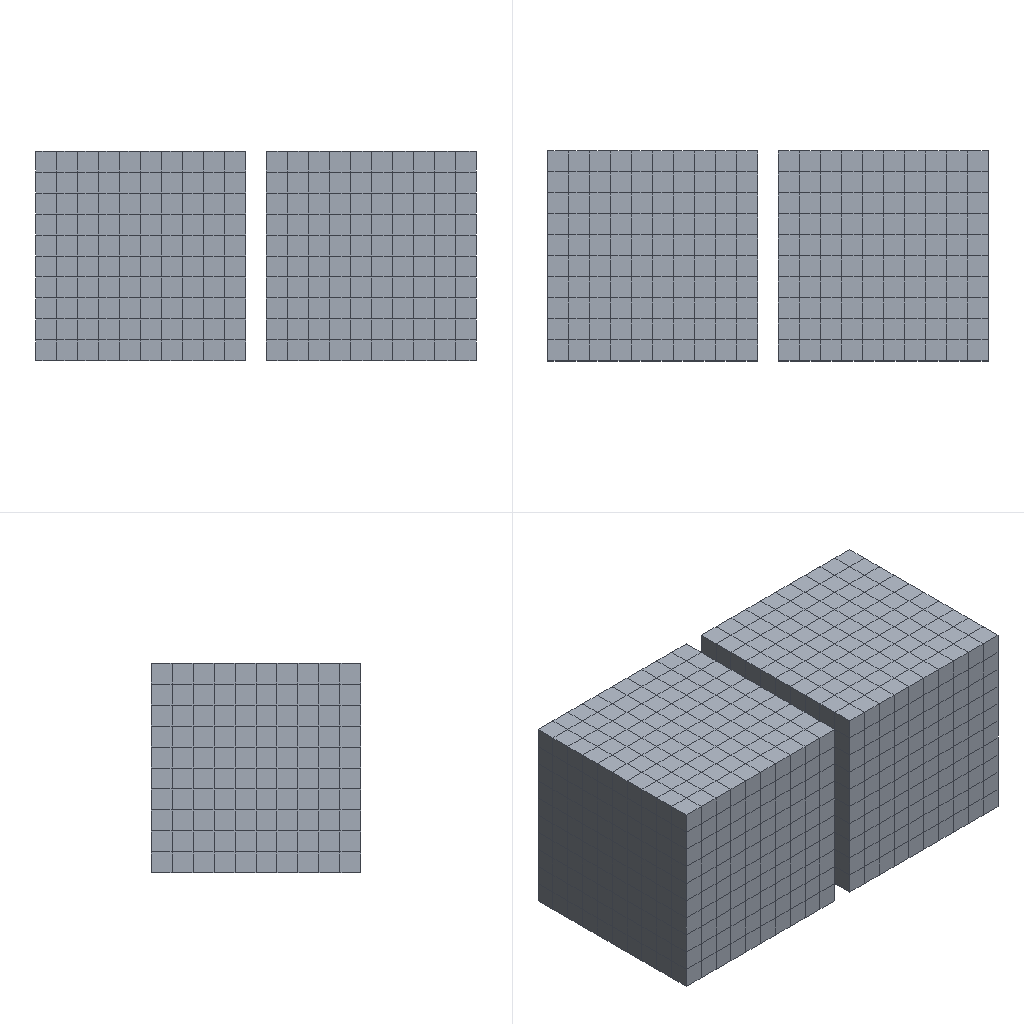Simulation study | abaqus
Set-up summary:
category,name,step,type,value,unit,region
solver,abaqus,,Abaqus/CAE 2024
units,SI m-kg-s (Pa),,inferred,E=3.45e+10 density=2550
analysis,Step-1,,frequency (modal),n_modes=10
mesh,nodes,,,2662
mesh,elements,,,2004
element_type,C3D8R,,,2000
element_type,CONN3D2,,,4
material,MATERIAL-1,,E,3.45e+10
material,MATERIAL-1,,nu,0.2
material,MATERIAL-1,,density,2550
material,MATERIAL-1,,behaviors,damping
material,MATERIAL-2,,E,3e+10
material,MATERIAL-2,,nu,0.3
material,MATERIAL-2,,density,2500
section,MATERIAL-2,,solid section,,,_PICKEDSET2
bc,Disp-BC-1,initial,encastre,[dofs=ENCASTRE],,_PICKEDSET37
constraint,connector section,,,1
Abaqus input file, long lists of numbers shortened:
*Heading
** Job name: deck Model name: 222
** Generated by: Abaqus/CAE 2024
*Preprint, echo=NO, model=NO, history=NO, contact=NO
**
** PARTS
**
*Part, name=PART-3
*Node
      1,          -5.,           0.,           5.
      2,          -5.,          0.5,           5.
** (1329 more lines like these left out)
*Element, type=C3D8R
   1,  122,  123,  134,  133,    1,    2,   13,   12
   2,  123,  124,  135,  134,    2,    3,   14,   13
** (998 more lines like these left out)
*Nset, nset=_PICKEDSET2, internal, generate
    1,  1331,     1
*Elset, elset=_PICKEDSET2, internal, generate
    1,  1000,     1
** Section: Section-1-_PICKEDSET2
*Solid Section, elset=_PICKEDSET2, material=MATERIAL-2
,
*End Part
**
**
** ASSEMBLY
**
*Assembly, name=Assembly
**
*Instance, name=PART-3-1, part=PART-3
*End Instance
**
*Instance, name=PART-3-2, part=PART-3
         5.5,           0.,           0.
*End Instance
**
*Element, type=CONN3D2
1, PART-3-1.122, PART-3-2.11
2, PART-3-1.133, PART-3-2.121
** (2 more lines like these left out)
*Connector Section, elset=_PickedSet21, behavior=ConnProp-1_CONNSECT-1
Cartesian, Cardan
"Datum csys-1",
*Nset, nset=SET-9, instance=PART-3-1
 1211, 1221, 1321, 1331
*Nset, nset=SET-9, instance=PART-3-2
   1,  11, 111, 121
*Nset, nset=WIRE-1-SET-3, instance=PART-3-1
 1211, 1221, 1321, 1331
*Nset, nset=WIRE-1-SET-3, instance=PART-3-2
   1,  11, 111, 121
*Nset, nset=_PICKEDSET32, internal, instance=PART-3-2, generate
 1211,  1331,     1
*Elset, elset=_PICKEDSET32, internal, instance=PART-3-2, generate
  901,  1000,     1
*Nset, nset=_PICKEDSET37, internal, instance=PART-3-2, generate
 1211,  1331,     1
*Elset, elset=_PICKEDSET37, internal, instance=PART-3-2, generate
  901,  1000,     1
*Elset, elset=_PickedSet21, internal, generate
 1,  4,  1
*Elset, elset=__PICKEDSURF33_S2, internal, instance=PART-3-1, generate
   1,  100,    1
*Surface, type=ELEMENT, name=_PICKEDSURF33, internal
__PICKEDSURF33_S2, S2
*Orientation, name="Datum csys-1"
          1.,           0.,           0.,           0.,           1.,           0.
1, 0.
*End Assembly
*Connector Behavior, name=ConnProp-1_CONNSECT-1
*Connector Elasticity, component=1
 5e+06,
*Connector Elasticity, component=2
 9e+09,
*Connector Elasticity, component=3
 6.9e+06,
**
** MATERIALS
**
*Material, name=MATERIAL-1
*Damping, alpha=0.516, beta=0.00077
*Density
2550.,
*Elastic
 3.45e+10, 0.2
*Material, name=MATERIAL-2
*Density
2500.,
*Elastic
 3e+10, 0.3
**
** BOUNDARY CONDITIONS
**
** Name: Disp-BC-1 Type: Symmetry/Antisymmetry/Encastre
*Boundary
_PICKEDSET37, ENCASTRE
** ----------------------------------------------------------------
**
** STEP: Step-1
**
*Step, name=Step-1, nlgeom=NO, perturbation
*Frequency, eigensolver=Lanczos, sim, acoustic coupling=on, normalization=mass
10, , , , ,
**
** OUTPUT REQUESTS
**
*Restart, write, frequency=0
**
** FIELD OUTPUT: F-Output-1
**
*Output, field
*Node Output
U,
*End Step
Results summary:
result,odb.job_status,,,JOB_STATUS_COMPLETED_SUCCESSFULLY,"consistent, unstated (Abaqus has no unit system)"
result,steps[0].procedure,Step-1,,*FREQUENCY,"consistent, unstated (Abaqus has no unit system)"
result,steps[0].time_period,Step-1,,0,"consistent, unstated (Abaqus has no unit system)"
result,steps[0].n_frames,Step-1,,11,"consistent, unstated (Abaqus has no unit system)"
result,steps[0].last_frame.id,Step-1,,1,"consistent, unstated (Abaqus has no unit system)"
result,steps[0].last_frame.value,Step-1,,10,"consistent, unstated (Abaqus has no unit system)"
result,steps[0].last_frame.description,Step-1,,Mode        10: Value =  6.75694E+05 Freq =   130.83     (cycles/time),"consistent, unstated (Abaqus has no unit system)"
result,steps[0].max_U_magnitude,Step-1,,0.003567,"consistent, unstated (Abaqus has no unit system)"
result,steps[0].eigenfrequencies_hz[1],Step-1,,0,"consistent, unstated (Abaqus has no unit system)"
result,steps[0].eigenfrequencies_hz[2],Step-1,,0,"consistent, unstated (Abaqus has no unit system)"
result,steps[0].eigenfrequencies_hz[3],Step-1,,0,"consistent, unstated (Abaqus has no unit system)"
result,steps[0].eigenfrequencies_hz[4],Step-1,,1.253,"consistent, unstated (Abaqus has no unit system)"
result,steps[0].eigenfrequencies_hz[5],Step-1,,1.522,"consistent, unstated (Abaqus has no unit system)"
result,steps[0].eigenfrequencies_hz[6],Step-1,,1.522,"consistent, unstated (Abaqus has no unit system)"
result,steps[0].eigenfrequencies_hz[7],Step-1,,73.26,"consistent, unstated (Abaqus has no unit system)"
result,steps[0].eigenfrequencies_hz[8],Step-1,,73.26,"consistent, unstated (Abaqus has no unit system)"
result,steps[0].eigenfrequencies_hz[9],Step-1,,98.617,"consistent, unstated (Abaqus has no unit system)"
result,steps[0].eigenfrequencies_hz[10],Step-1,,130.83,"consistent, unstated (Abaqus has no unit system)"